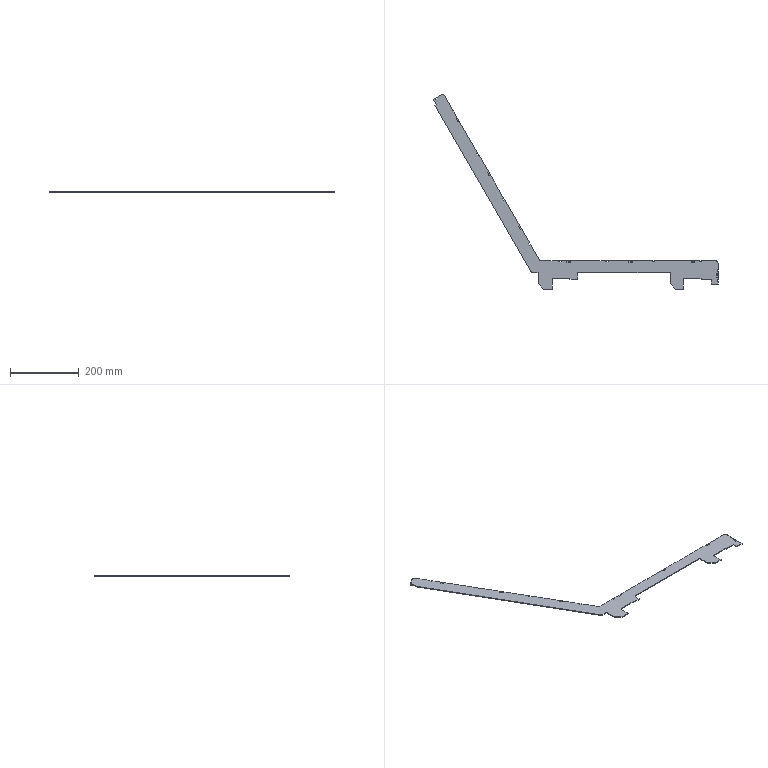Part | STEP file | zh002-1 | 1 solid | 108 faces | box 824.943 x 563.765 x 2 mm | volume 93562 mm3 | plane 104 | cylinder 4 | commonest cylinder face diameters 20 x3 8 x1